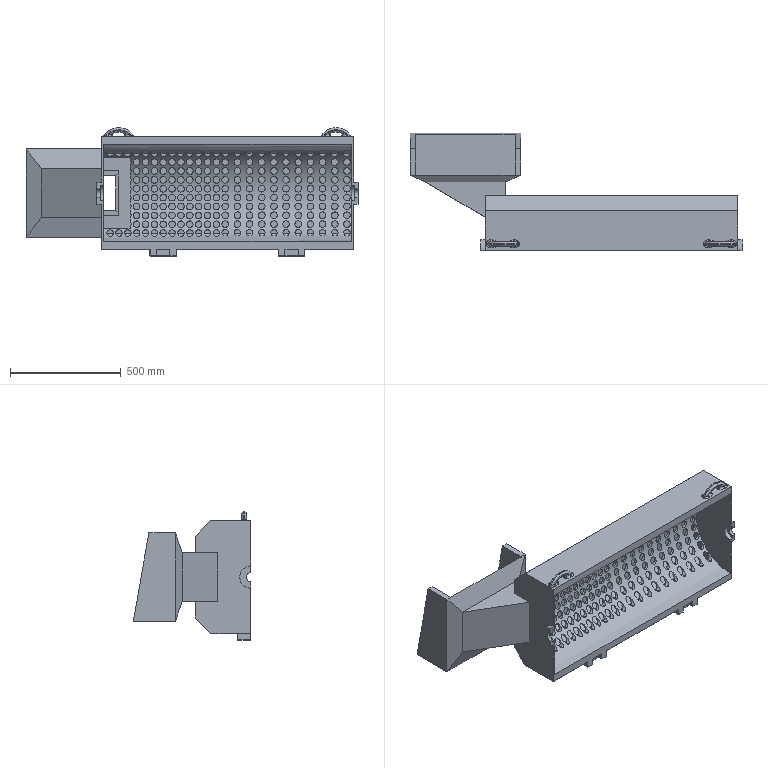Part | SolidWorks | 1 solid | 640 faces | box 1500 x 530.531 x 580 mm | volume 26783314 mm3 | cylinder 474 | plane 134 | spline 24 | torus 8 | commonest cylinder face diameters 30 x440 16 x14 10 x8 40 x2 68 x2 100 x2